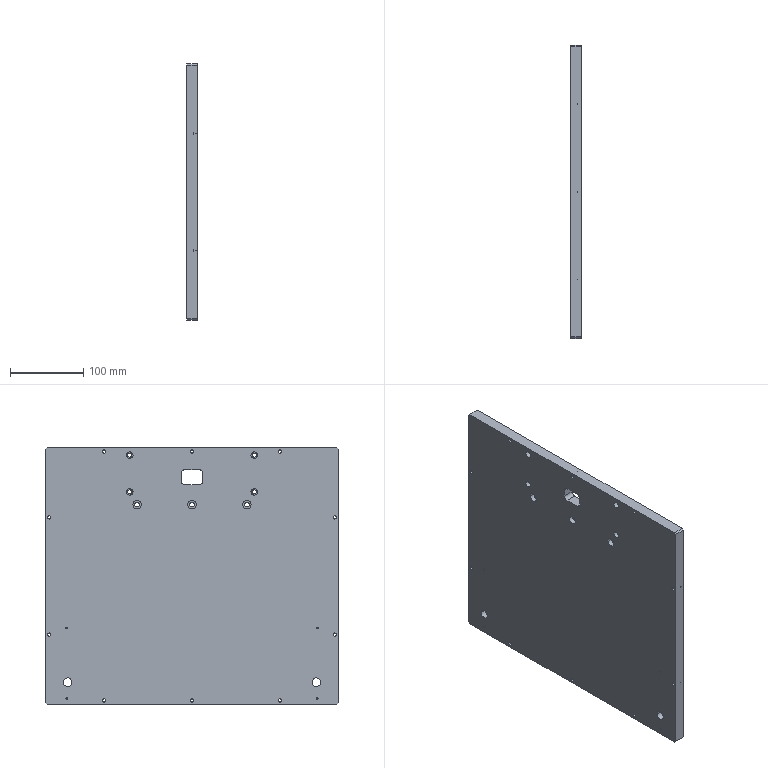Part | STEP file | PN_0002 | 1 solid | 132 faces | box 15 x 400 x 350 mm | volume 2071753 mm3 | cylinder 96 | plane 36 | commonest cylinder face diameters 4.5 x20 7.5 x20 2.5 x8 3 x8 5.5 x8 9 x8